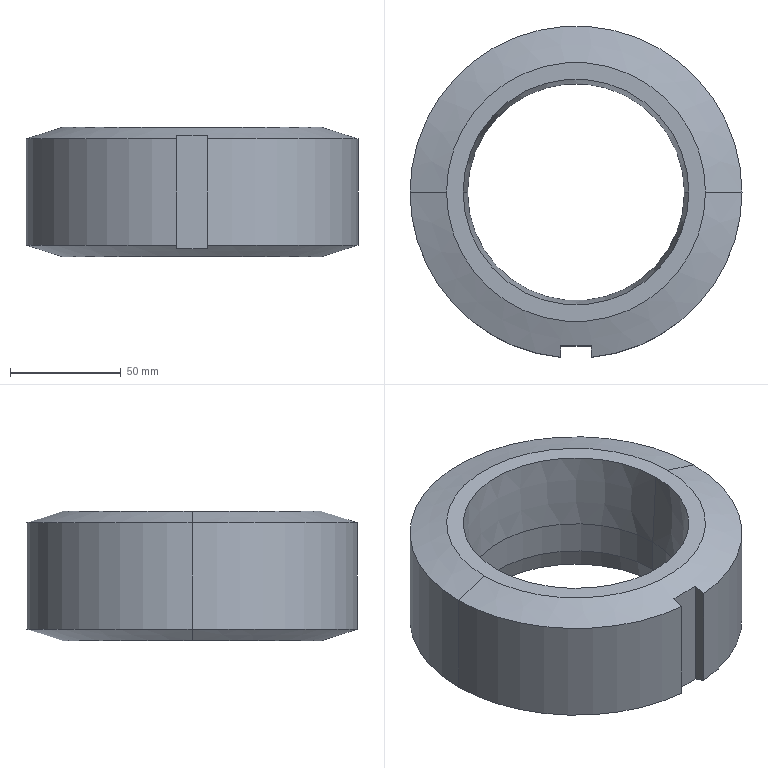Part | SolidWorks | features BaseBody 1, ICE 1 | 1 solid | 18 faces | box 150 x 149.673 x 58.5 mm | volume 537765 mm3 | cone 8 | cylinder 5 | plane 5 | commonest cylinder face diameters 150 x3 98 x2
STEP:
#1=CARTESIAN_POINT('',(570.231,234.744,-789.693));
#2=VERTEX_POINT('',#1);
#3=CARTESIAN_POINT('',(472.231,234.744,-789.693));
#4=VERTEX_POINT('',#3);
#5=CARTESIAN_POINT('',(521.231,234.744,-789.693));
#6=DIRECTION('',(0.,0.,-1.));
#7=DIRECTION('',(-1.,0.,0.));
#8=AXIS2_PLACEMENT_3D('',#5,#6,#7);
#9=CIRCLE('',#8,49.);
#10=EDGE_CURVE('',#2,#4,#9,.T.);
#11=ORIENTED_EDGE('',*,*,#10,.T.);
#12=CARTESIAN_POINT('',(470.231,234.744,-754.693));
#13=VERTEX_POINT('',#12);
#14=CARTESIAN_POINT('',(470.231,234.744,-754.693));
#15=DIRECTION('',(-0.05705,0.,0.9984));
#16=VECTOR('',#15,1000.);
#17=LINE('',#14,#16);
#18=EDGE_CURVE('',#4,#13,#17,.T.);
#19=ORIENTED_EDGE('',*,*,#18,.T.);
#20=CARTESIAN_POINT('',(572.231,234.744,-754.693));
#21=VERTEX_POINT('',#20);
#22=CARTESIAN_POINT('',(521.231,234.744,-754.693));
#23=DIRECTION('',(0.,0.,-1.));
#24=DIRECTION('',(-1.,0.,0.));
#25=AXIS2_PLACEMENT_3D('',#22,#23,#24);
#26=CIRCLE('',#25,51.);
#27=EDGE_CURVE('',#21,#13,#26,.T.);
#28=ORIENTED_EDGE('',*,*,#27,.F.);
#29=CARTESIAN_POINT('',(572.231,234.744,-754.693));
#30=DIRECTION('',(0.05705,0.,0.9984));
#31=VECTOR('',#30,1000.);
#32=LINE('',#29,#31);
#33=EDGE_CURVE('',#2,#21,#32,.T.);
#34=ORIENTED_EDGE('',*,*,#33,.F.);
#35=EDGE_LOOP('',(#11,#19,#28,#34));
#36=FACE_OUTER_BOUND('',#35,.T.);
#37=CARTESIAN_POINT('',(521.231,234.744,-754.693));
#38=DIRECTION('',(0.,0.,1.));
#39=DIRECTION('',(1.,0.,0.));
#40=AXIS2_PLACEMENT_3D('',#37,#38,#39);
#41=CONICAL_SURFACE('',#40,51.,0.05708);
#42=ADVANCED_FACE('',(#36),#41,.F.);
#43=CARTESIAN_POINT('',(462.731,234.744,-754.693));
#44=VERTEX_POINT('',#43);
#45=CARTESIAN_POINT('',(579.731,234.744,-754.693));
#46=VERTEX_POINT('',#45);
#47=CARTESIAN_POINT('',(521.231,234.744,-754.693));
#48=DIRECTION('',(0.,0.,-1.));
#49=DIRECTION('',(-1.,0.,0.));
#50=AXIS2_PLACEMENT_3D('',#47,#48,#49);
#51=CIRCLE('',#50,58.5);
#52=EDGE_CURVE('',#44,#46,#51,.T.);
#53=ORIENTED_EDGE('',*,*,#52,.T.);
#54=CARTESIAN_POINT('',(596.231,234.744,-759.943));
#55=VERTEX_POINT('',#54);
#56=CARTESIAN_POINT('',(579.731,234.744,-754.693));
#57=DIRECTION('',(0.9529,0.,-0.3032));
#58=VECTOR('',#57,1000.);
#59=LINE('',#56,#58);
#60=EDGE_CURVE('',#46,#55,#59,.T.);
#61=ORIENTED_EDGE('',*,*,#60,.T.);
#62=CARTESIAN_POINT('',(446.231,234.744,-759.943));
#63=VERTEX_POINT('',#62);
#64=CARTESIAN_POINT('',(521.231,234.744,-759.943));
#65=DIRECTION('',(0.,0.,-1.));
#66=DIRECTION('',(-1.,0.,0.));
#67=AXIS2_PLACEMENT_3D('',#64,#65,#66);
#68=CIRCLE('',#67,75.);
#69=EDGE_CURVE('',#63,#55,#68,.T.);
#70=ORIENTED_EDGE('',*,*,#69,.F.);
#71=CARTESIAN_POINT('',(462.731,234.744,-754.693));
#72=DIRECTION('',(-0.9529,0.,-0.3032));
#73=VECTOR('',#72,1000.);
#74=LINE('',#71,#73);
#75=EDGE_CURVE('',#44,#63,#74,.T.);
#76=ORIENTED_EDGE('',*,*,#75,.F.);
#77=EDGE_LOOP('',(#53,#61,#70,#76));
#78=FACE_OUTER_BOUND('',#77,.T.);
#79=CARTESIAN_POINT('',(521.231,234.744,-754.693));
#80=DIRECTION('',(0.,0.,-1.));
#81=DIRECTION('',(-1.,0.,0.));
#82=AXIS2_PLACEMENT_3D('',#79,#80,#81);
#83=CONICAL_SURFACE('',#82,58.5,1.263);
#84=ADVANCED_FACE('',(#78),#83,.T.);
#85=CARTESIAN_POINT('',(462.731,234.744,-813.193));
#86=VERTEX_POINT('',#85);
#87=CARTESIAN_POINT('',(579.731,234.744,-813.193));
#88=VERTEX_POINT('',#87);
#89=CARTESIAN_POINT('',(521.231,234.744,-813.193));
#90=DIRECTION('',(0.,0.,-1.));
#91=DIRECTION('',(-1.,0.,0.));
#92=AXIS2_PLACEMENT_3D('',#89,#90,#91);
#93=CIRCLE('',#92,58.5);
#94=EDGE_CURVE('',#86,#88,#93,.T.);
#95=ORIENTED_EDGE('',*,*,#94,.F.);
#96=CARTESIAN_POINT('',(446.231,234.744,-807.943));
#97=VERTEX_POINT('',#96);
#98=CARTESIAN_POINT('',(462.731,234.744,-813.193));
#99=DIRECTION('',(-0.9529,0.,0.3032));
#100=VECTOR('',#99,1000.);
#101=LINE('',#98,#100);
#102=EDGE_CURVE('',#86,#97,#101,.T.);
#103=ORIENTED_EDGE('',*,*,#102,.T.);
#104=CARTESIAN_POINT('',(596.231,234.744,-807.943));
#105=VERTEX_POINT('',#104);
#106=CARTESIAN_POINT('',(521.231,234.744,-807.943));
#107=DIRECTION('',(0.,0.,-1.));
#108=DIRECTION('',(-1.,0.,0.));
#109=AXIS2_PLACEMENT_3D('',#106,#107,#108);
#110=CIRCLE('',#109,75.);
#111=EDGE_CURVE('',#97,#105,#110,.T.);
#112=ORIENTED_EDGE('',*,*,#111,.T.);
#113=CARTESIAN_POINT('',(579.731,234.744,-813.193));
#114=DIRECTION('',(0.9529,0.,0.3032));
#115=VECTOR('',#114,1000.);
#116=LINE('',#113,#115);
#117=EDGE_CURVE('',#88,#105,#116,.T.);
#118=ORIENTED_EDGE('',*,*,#117,.F.);
#119=EDGE_LOOP('',(#95,#103,#112,#118));
#120=FACE_OUTER_BOUND('',#119,.T.);
#121=CARTESIAN_POINT('',(521.231,234.744,-813.193));
#122=DIRECTION('',(0.,0.,1.));
#123=DIRECTION('',(1.,0.,0.));
#124=AXIS2_PLACEMENT_3D('',#121,#122,#123);
#125=CONICAL_SURFACE('',#124,58.5,1.263);
#126=ADVANCED_FACE('',(#120),#125,.T.);
#127=ORIENTED_EDGE('',*,*,#111,.F.);
#128=CARTESIAN_POINT('',(446.231,234.744,-814.693));
#129=DIRECTION('',(0.,0.,1.));
#130=VECTOR('',#129,1000.);
#131=LINE('',#128,#130);
#132=EDGE_CURVE('',#97,#63,#131,.T.);
#133=ORIENTED_EDGE('',*,*,#132,.T.);
#134=ORIENTED_EDGE('',*,*,#69,.T.);
#135=CARTESIAN_POINT('',(596.231,234.744,-814.693));
#136=DIRECTION('',(0.,0.,1.));
#137=VECTOR('',#136,1000.);
#138=LINE('',#135,#137);
#139=EDGE_CURVE('',#105,#55,#138,.T.);
#140=ORIENTED_EDGE('',*,*,#139,.F.);
#141=EDGE_LOOP('',(#127,#133,#134,#140));
#142=FACE_OUTER_BOUND('',#141,.T.);
#143=CARTESIAN_POINT('',(521.231,234.744,-814.693));
#144=DIRECTION('',(0.,0.,1.));
#145=DIRECTION('',(1.,0.,0.));
#146=AXIS2_PLACEMENT_3D('',#143,#144,#145);
#147=CYLINDRICAL_SURFACE('',#146,75.);
#148=ADVANCED_FACE('',(#142),#147,.T.);
#149=CARTESIAN_POINT('',(528.231,160.071,-807.943));
#150=VERTEX_POINT('',#149);
#151=CARTESIAN_POINT('',(521.231,234.744,-807.943));
#152=DIRECTION('',(0.,0.,-1.));
#153=DIRECTION('',(-1.,0.,0.));
#154=AXIS2_PLACEMENT_3D('',#151,#152,#153);
#155=CIRCLE('',#154,75.);
#156=EDGE_CURVE('',#105,#150,#155,.T.);
#157=ORIENTED_EDGE('',*,*,#156,.F.);
#158=ORIENTED_EDGE('',*,*,#139,.T.);
#159=CARTESIAN_POINT('',(528.231,160.071,-759.943));
#160=VERTEX_POINT('',#159);
#161=CARTESIAN_POINT('',(521.231,234.744,-759.943));
#162=DIRECTION('',(0.,0.,-1.));
#163=DIRECTION('',(-1.,0.,0.));
#164=AXIS2_PLACEMENT_3D('',#161,#162,#163);
#165=CIRCLE('',#164,75.);
#166=EDGE_CURVE('',#55,#160,#165,.T.);
#167=ORIENTED_EDGE('',*,*,#166,.T.);
#168=CARTESIAN_POINT('',(528.231,160.071,-814.693));
#169=DIRECTION('',(0.,0.,-1.));
#170=VECTOR('',#169,1000.);
#171=LINE('',#168,#170);
#172=EDGE_CURVE('',#160,#150,#171,.T.);
#173=ORIENTED_EDGE('',*,*,#172,.T.);
#174=EDGE_LOOP('',(#157,#158,#167,#173));
#175=FACE_OUTER_BOUND('',#174,.T.);
#176=CARTESIAN_POINT('',(521.231,234.744,-814.693));
#177=DIRECTION('',(0.,0.,1.));
#178=DIRECTION('',(1.,0.,0.));
#179=AXIS2_PLACEMENT_3D('',#176,#177,#178);
#180=CYLINDRICAL_SURFACE('',#179,75.);
#181=ADVANCED_FACE('',(#175),#180,.T.);
#182=ORIENTED_EDGE('',*,*,#10,.F.);
#183=CARTESIAN_POINT('',(570.231,234.744,-804.693));
#184=VERTEX_POINT('',#183);
#185=CARTESIAN_POINT('',(570.231,234.744,-754.693));
#186=DIRECTION('',(0.,0.,-1.));
#187=VECTOR('',#186,1000.);
#188=LINE('',#185,#187);
#189=EDGE_CURVE('',#2,#184,#188,.T.);
#190=ORIENTED_EDGE('',*,*,#189,.T.);
#191=CARTESIAN_POINT('',(472.231,234.744,-804.693));
#192=VERTEX_POINT('',#191);
#193=CARTESIAN_POINT('',(521.231,234.744,-804.693));
#194=DIRECTION('',(0.,0.,-1.));
#195=DIRECTION('',(-1.,0.,0.));
#196=AXIS2_PLACEMENT_3D('',#193,#194,#195);
#197=CIRCLE('',#196,49.);
#198=EDGE_CURVE('',#184,#192,#197,.T.);
#199=ORIENTED_EDGE('',*,*,#198,.T.);
#200=CARTESIAN_POINT('',(472.231,234.744,-754.693));
#201=DIRECTION('',(0.,0.,-1.));
#202=VECTOR('',#201,1000.);
#203=LINE('',#200,#202);
#204=EDGE_CURVE('',#4,#192,#203,.T.);
#205=ORIENTED_EDGE('',*,*,#204,.F.);
#206=EDGE_LOOP('',(#182,#190,#199,#205));
#207=FACE_OUTER_BOUND('',#206,.T.);
#208=CARTESIAN_POINT('',(521.231,234.744,-754.693));
#209=DIRECTION('',(0.,0.,-1.));
#210=DIRECTION('',(-1.,0.,0.));
#211=AXIS2_PLACEMENT_3D('',#208,#209,#210);
#212=CYLINDRICAL_SURFACE('',#211,49.);
#213=ADVANCED_FACE('',(#207),#212,.F.);
#214=ORIENTED_EDGE('',*,*,#198,.F.);
#215=CARTESIAN_POINT('',(571.931,234.744,-813.193));
#216=VERTEX_POINT('',#215);
#217=CARTESIAN_POINT('',(570.231,234.744,-804.693));
#218=DIRECTION('',(0.1961,0.,-0.9806));
#219=VECTOR('',#218,1000.);
#220=LINE('',#217,#219);
#221=EDGE_CURVE('',#184,#216,#220,.T.);
#222=ORIENTED_EDGE('',*,*,#221,.T.);
#223=CARTESIAN_POINT('',(470.531,234.744,-813.193));
#224=VERTEX_POINT('',#223);
#225=CARTESIAN_POINT('',(521.231,234.744,-813.193));
#226=DIRECTION('',(0.,0.,-1.));
#227=DIRECTION('',(-1.,0.,0.));
#228=AXIS2_PLACEMENT_3D('',#225,#226,#227);
#229=CIRCLE('',#228,50.7);
#230=EDGE_CURVE('',#216,#224,#229,.T.);
#231=ORIENTED_EDGE('',*,*,#230,.T.);
#232=CARTESIAN_POINT('',(472.231,234.744,-804.693));
#233=DIRECTION('',(-0.1961,0.,-0.9806));
#234=VECTOR('',#233,1000.);
#235=LINE('',#232,#234);
#236=EDGE_CURVE('',#192,#224,#235,.T.);
#237=ORIENTED_EDGE('',*,*,#236,.F.);
#238=EDGE_LOOP('',(#214,#222,#231,#237));
#239=FACE_OUTER_BOUND('',#238,.T.);
#240=CARTESIAN_POINT('',(521.231,234.744,-804.693));
#241=DIRECTION('',(0.,0.,-1.));
#242=DIRECTION('',(-1.,0.,0.));
#243=AXIS2_PLACEMENT_3D('',#240,#241,#242);
#244=CONICAL_SURFACE('',#243,49.,0.1974);
#245=ADVANCED_FACE('',(#239),#244,.F.);
#246=ORIENTED_EDGE('',*,*,#221,.F.);
#247=CARTESIAN_POINT('',(521.231,234.744,-804.693));
#248=DIRECTION('',(0.,0.,-1.));
#249=DIRECTION('',(-1.,0.,0.));
#250=AXIS2_PLACEMENT_3D('',#247,#248,#249);
#251=CIRCLE('',#250,49.);
#252=EDGE_CURVE('',#192,#184,#251,.T.);
#253=ORIENTED_EDGE('',*,*,#252,.F.);
#254=ORIENTED_EDGE('',*,*,#236,.T.);
#255=CARTESIAN_POINT('',(521.231,234.744,-813.193));
#256=DIRECTION('',(0.,0.,-1.));
#257=DIRECTION('',(-1.,0.,0.));
#258=AXIS2_PLACEMENT_3D('',#255,#256,#257);
#259=CIRCLE('',#258,50.7);
#260=EDGE_CURVE('',#224,#216,#259,.T.);
#261=ORIENTED_EDGE('',*,*,#260,.T.);
#262=EDGE_LOOP('',(#246,#253,#254,#261));
#263=FACE_OUTER_BOUND('',#262,.T.);
#264=CARTESIAN_POINT('',(521.231,234.744,-804.693));
#265=DIRECTION('',(0.,0.,-1.));
#266=DIRECTION('',(-1.,0.,0.));
#267=AXIS2_PLACEMENT_3D('',#264,#265,#266);
#268=CONICAL_SURFACE('',#267,49.,0.1974);
#269=ADVANCED_FACE('',(#263),#268,.F.);
#270=ORIENTED_EDGE('',*,*,#189,.F.);
#271=CARTESIAN_POINT('',(521.231,234.744,-789.693));
#272=DIRECTION('',(0.,0.,-1.));
#273=DIRECTION('',(-1.,0.,0.));
#274=AXIS2_PLACEMENT_3D('',#271,#272,#273);
#275=CIRCLE('',#274,49.);
#276=EDGE_CURVE('',#4,#2,#275,.T.);
#277=ORIENTED_EDGE('',*,*,#276,.F.);
#278=ORIENTED_EDGE('',*,*,#204,.T.);
#279=ORIENTED_EDGE('',*,*,#252,.T.);
#280=EDGE_LOOP('',(#270,#277,#278,#279));
#281=FACE_OUTER_BOUND('',#280,.T.);
#282=CARTESIAN_POINT('',(521.231,234.744,-754.693));
#283=DIRECTION('',(0.,0.,-1.));
#284=DIRECTION('',(-1.,0.,0.));
#285=AXIS2_PLACEMENT_3D('',#282,#283,#284);
#286=CYLINDRICAL_SURFACE('',#285,49.);
#287=ADVANCED_FACE('',(#281),#286,.F.);
#288=ORIENTED_EDGE('',*,*,#27,.T.);
#289=CARTESIAN_POINT('',(521.231,234.744,-754.693));
#290=DIRECTION('',(0.,0.,-1.));
#291=DIRECTION('',(-1.,0.,0.));
#292=AXIS2_PLACEMENT_3D('',#289,#290,#291);
#293=CIRCLE('',#292,51.);
#294=EDGE_CURVE('',#13,#21,#293,.T.);
#295=ORIENTED_EDGE('',*,*,#294,.T.);
#296=EDGE_LOOP('',(#288,#295));
#297=FACE_BOUND('',#296,.T.);
#298=ORIENTED_EDGE('',*,*,#52,.F.);
#299=CARTESIAN_POINT('',(521.231,234.744,-754.693));
#300=DIRECTION('',(0.,0.,-1.));
#301=DIRECTION('',(-1.,0.,0.));
#302=AXIS2_PLACEMENT_3D('',#299,#300,#301);
#303=CIRCLE('',#302,58.5);
#304=EDGE_CURVE('',#46,#44,#303,.T.);
#305=ORIENTED_EDGE('',*,*,#304,.F.);
#306=EDGE_LOOP('',(#298,#305));
#307=FACE_OUTER_BOUND('',#306,.T.);
#308=CARTESIAN_POINT('',(521.231,234.744,-754.693));
#309=DIRECTION('',(0.,0.,-1.));
#310=DIRECTION('',(-1.,0.,0.));
#311=AXIS2_PLACEMENT_3D('',#308,#309,#310);
#312=PLANE('',#311);
#313=ADVANCED_FACE('',(#297,#307),#312,.F.);
#314=ORIENTED_EDGE('',*,*,#132,.F.);
#315=CARTESIAN_POINT('',(514.231,160.071,-807.943));
#316=VERTEX_POINT('',#315);
#317=CARTESIAN_POINT('',(521.231,234.744,-807.943));
#318=DIRECTION('',(0.,0.,-1.));
#319=DIRECTION('',(-1.,0.,0.));
#320=AXIS2_PLACEMENT_3D('',#317,#318,#319);
#321=CIRCLE('',#320,75.);
#322=EDGE_CURVE('',#316,#97,#321,.T.);
#323=ORIENTED_EDGE('',*,*,#322,.F.);
#324=CARTESIAN_POINT('',(514.231,160.071,-759.943));
#325=VERTEX_POINT('',#324);
#326=CARTESIAN_POINT('',(514.231,160.071,-814.693));
#327=DIRECTION('',(0.,0.,1.));
#328=VECTOR('',#327,1000.);
#329=LINE('',#326,#328);
#330=EDGE_CURVE('',#316,#325,#329,.T.);
#331=ORIENTED_EDGE('',*,*,#330,.T.);
#332=CARTESIAN_POINT('',(521.231,234.744,-759.943));
#333=DIRECTION('',(0.,0.,-1.));
#334=DIRECTION('',(-1.,0.,0.));
#335=AXIS2_PLACEMENT_3D('',#332,#333,#334);
#336=CIRCLE('',#335,75.);
#337=EDGE_CURVE('',#325,#63,#336,.T.);
#338=ORIENTED_EDGE('',*,*,#337,.T.);
#339=EDGE_LOOP('',(#314,#323,#331,#338));
#340=FACE_OUTER_BOUND('',#339,.T.);
#341=CARTESIAN_POINT('',(521.231,234.744,-814.693));
#342=DIRECTION('',(0.,0.,1.));
#343=DIRECTION('',(1.,0.,0.));
#344=AXIS2_PLACEMENT_3D('',#341,#342,#343);
#345=CYLINDRICAL_SURFACE('',#344,75.);
#346=ADVANCED_FACE('',(#340),#345,.T.);
#347=ORIENTED_EDGE('',*,*,#102,.F.);
#348=CARTESIAN_POINT('',(521.231,234.744,-813.193));
#349=DIRECTION('',(0.,0.,-1.));
#350=DIRECTION('',(-1.,0.,0.));
#351=AXIS2_PLACEMENT_3D('',#348,#349,#350);
#352=CIRCLE('',#351,58.5);
#353=EDGE_CURVE('',#88,#86,#352,.T.);
#354=ORIENTED_EDGE('',*,*,#353,.F.);
#355=ORIENTED_EDGE('',*,*,#117,.T.);
#356=ORIENTED_EDGE('',*,*,#156,.T.);
#357=CARTESIAN_POINT('',(528.231,165.244,-809.581));
#358=VERTEX_POINT('',#357);
#359=CARTESIAN_POINT('',(528.231,165.244,-809.581));
#360=CARTESIAN_POINT('',(528.231,163.692,-809.09));
#361=CARTESIAN_POINT('',(528.231,162.14,-808.598));
#362=CARTESIAN_POINT('',(528.231,160.588,-808.107));
#363=CARTESIAN_POINT('',(528.231,160.415,-808.052));
#364=CARTESIAN_POINT('',(528.231,160.243,-807.997));
#365=CARTESIAN_POINT('',(528.231,160.071,-807.943));
#366=B_SPLINE_CURVE_WITH_KNOTS('',3,(#359,#360,#361,#362,#363,#364,#365),.UNSPECIFIED.,.F.,.F.,(4,3,4),(0.008941,0.01383,0.01437),.UNSPECIFIED.);
#367=EDGE_CURVE('',#358,#150,#366,.T.);
#368=ORIENTED_EDGE('',*,*,#367,.F.);
#369=CARTESIAN_POINT('',(514.231,165.244,-809.581));
#370=VERTEX_POINT('',#369);
#371=CARTESIAN_POINT('',(514.231,165.244,-809.581));
#372=CARTESIAN_POINT('',(516.561,165.244,-809.655));
#373=CARTESIAN_POINT('',(518.893,165.244,-809.693));
#374=CARTESIAN_POINT('',(523.56,165.244,-809.693));
#375=CARTESIAN_POINT('',(525.896,165.244,-809.656));
#376=CARTESIAN_POINT('',(528.231,165.244,-809.581));
#377=B_SPLINE_CURVE_WITH_KNOTS('',3,(#371,#372,#373,#374,#375,#376),.UNSPECIFIED.,.F.,.F.,(4,2,4),(0.01756,0.02456,0.03155),.UNSPECIFIED.);
#378=EDGE_CURVE('',#370,#358,#377,.T.);
#379=ORIENTED_EDGE('',*,*,#378,.F.);
#380=CARTESIAN_POINT('',(514.231,160.071,-807.943));
#381=CARTESIAN_POINT('',(514.231,160.243,-807.997));
#382=CARTESIAN_POINT('',(514.231,160.415,-808.052));
#383=CARTESIAN_POINT('',(514.231,160.588,-808.107));
#384=CARTESIAN_POINT('',(514.231,162.14,-808.598));
#385=CARTESIAN_POINT('',(514.231,163.692,-809.09));
#386=CARTESIAN_POINT('',(514.231,165.244,-809.581));
#387=B_SPLINE_CURVE_WITH_KNOTS('',3,(#380,#381,#382,#383,#384,#385,#386),.UNSPECIFIED.,.F.,.F.,(4,3,4),(0.01328,0.01383,0.01871),.UNSPECIFIED.);
#388=EDGE_CURVE('',#316,#370,#387,.T.);
#389=ORIENTED_EDGE('',*,*,#388,.F.);
#390=ORIENTED_EDGE('',*,*,#322,.T.);
#391=EDGE_LOOP('',(#347,#354,#355,#356,#368,#379,#389,#390));
#392=FACE_OUTER_BOUND('',#391,.T.);
#393=CARTESIAN_POINT('',(521.231,234.744,-813.193));
#394=DIRECTION('',(0.,0.,1.));
#395=DIRECTION('',(1.,0.,0.));
#396=AXIS2_PLACEMENT_3D('',#393,#394,#395);
#397=CONICAL_SURFACE('',#396,58.5,1.263);
#398=ADVANCED_FACE('',(#392),#397,.T.);
#399=ORIENTED_EDGE('',*,*,#60,.F.);
#400=ORIENTED_EDGE('',*,*,#304,.T.);
#401=ORIENTED_EDGE('',*,*,#75,.T.);
#402=ORIENTED_EDGE('',*,*,#337,.F.);
#403=CARTESIAN_POINT('',(514.231,165.244,-758.305));
#404=VERTEX_POINT('',#403);
#405=CARTESIAN_POINT('',(514.231,160.071,-759.943));
#406=CARTESIAN_POINT('',(514.231,160.243,-759.888));
#407=CARTESIAN_POINT('',(514.231,160.415,-759.834));
#408=CARTESIAN_POINT('',(514.231,160.588,-759.779));
#409=CARTESIAN_POINT('',(514.231,162.14,-759.288));
#410=CARTESIAN_POINT('',(514.231,163.692,-758.796));
#411=CARTESIAN_POINT('',(514.231,165.244,-758.305));
#412=B_SPLINE_CURVE_WITH_KNOTS('',3,(#405,#406,#407,#408,#409,#410,#411),.UNSPECIFIED.,.F.,.F.,(4,3,4),(0.01328,0.01383,0.01871),.UNSPECIFIED.);
#413=EDGE_CURVE('',#325,#404,#412,.T.);
#414=ORIENTED_EDGE('',*,*,#413,.T.);
#415=CARTESIAN_POINT('',(528.231,165.244,-758.305));
#416=VERTEX_POINT('',#415);
#417=CARTESIAN_POINT('',(514.231,165.244,-758.305));
#418=CARTESIAN_POINT('',(516.561,165.244,-758.231));
#419=CARTESIAN_POINT('',(518.893,165.244,-758.193));
#420=CARTESIAN_POINT('',(523.56,165.244,-758.193));
#421=CARTESIAN_POINT('',(525.896,165.244,-758.23));
#422=CARTESIAN_POINT('',(528.231,165.244,-758.305));
#423=B_SPLINE_CURVE_WITH_KNOTS('',3,(#417,#418,#419,#420,#421,#422),.UNSPECIFIED.,.F.,.F.,(4,2,4),(0.01756,0.02456,0.03155),.UNSPECIFIED.);
#424=EDGE_CURVE('',#404,#416,#423,.T.);
#425=ORIENTED_EDGE('',*,*,#424,.T.);
#426=CARTESIAN_POINT('',(528.231,165.244,-758.305));
#427=CARTESIAN_POINT('',(528.231,163.692,-758.796));
#428=CARTESIAN_POINT('',(528.231,162.14,-759.288));
#429=CARTESIAN_POINT('',(528.231,160.588,-759.779));
#430=CARTESIAN_POINT('',(528.231,160.415,-759.834));
#431=CARTESIAN_POINT('',(528.231,160.243,-759.888));
#432=CARTESIAN_POINT('',(528.231,160.071,-759.943));
#433=B_SPLINE_CURVE_WITH_KNOTS('',3,(#426,#427,#428,#429,#430,#431,#432),.UNSPECIFIED.,.F.,.F.,(4,3,4),(0.008941,0.01383,0.01437),.UNSPECIFIED.);
#434=EDGE_CURVE('',#416,#160,#433,.T.);
#435=ORIENTED_EDGE('',*,*,#434,.T.);
#436=ORIENTED_EDGE('',*,*,#166,.F.);
#437=EDGE_LOOP('',(#399,#400,#401,#402,#414,#425,#435,#436));
#438=FACE_OUTER_BOUND('',#437,.T.);
#439=CARTESIAN_POINT('',(521.231,234.744,-754.693));
#440=DIRECTION('',(0.,0.,-1.));
#441=DIRECTION('',(-1.,0.,0.));
#442=AXIS2_PLACEMENT_3D('',#439,#440,#441);
#443=CONICAL_SURFACE('',#442,58.5,1.263);
#444=ADVANCED_FACE('',(#438),#443,.T.);
#445=ORIENTED_EDGE('',*,*,#18,.F.);
#446=ORIENTED_EDGE('',*,*,#276,.T.);
#447=ORIENTED_EDGE('',*,*,#33,.T.);
#448=ORIENTED_EDGE('',*,*,#294,.F.);
#449=EDGE_LOOP('',(#445,#446,#447,#448));
#450=FACE_OUTER_BOUND('',#449,.T.);
#451=CARTESIAN_POINT('',(521.231,234.744,-754.693));
#452=DIRECTION('',(0.,0.,1.));
#453=DIRECTION('',(1.,0.,0.));
#454=AXIS2_PLACEMENT_3D('',#451,#452,#453);
#455=CONICAL_SURFACE('',#454,51.,0.05708);
#456=ADVANCED_FACE('',(#450),#455,.F.);
#457=ORIENTED_EDGE('',*,*,#378,.T.);
#458=CARTESIAN_POINT('',(528.231,165.244,-1254.693));
#459=DIRECTION('',(0.,0.,1.));
#460=VECTOR('',#459,1000.);
#461=LINE('',#458,#460);
#462=EDGE_CURVE('',#358,#416,#461,.T.);
#463=ORIENTED_EDGE('',*,*,#462,.T.);
#464=ORIENTED_EDGE('',*,*,#424,.F.);
#465=CARTESIAN_POINT('',(514.231,165.244,-1254.693));
#466=DIRECTION('',(0.,0.,1.));
#467=VECTOR('',#466,1000.);
#468=LINE('',#465,#467);
#469=EDGE_CURVE('',#370,#404,#468,.T.);
#470=ORIENTED_EDGE('',*,*,#469,.F.);
#471=EDGE_LOOP('',(#457,#463,#464,#470));
#472=FACE_OUTER_BOUND('',#471,.T.);
#473=CARTESIAN_POINT('',(528.231,165.244,-1254.693));
#474=DIRECTION('',(0.,1.,0.));
#475=DIRECTION('',(0.,0.,-1.));
#476=AXIS2_PLACEMENT_3D('',#473,#474,#475);
#477=PLANE('',#476);
#478=ADVANCED_FACE('',(#472),#477,.F.);
#479=ORIENTED_EDGE('',*,*,#367,.T.);
#480=ORIENTED_EDGE('',*,*,#172,.F.);
#481=ORIENTED_EDGE('',*,*,#434,.F.);
#482=ORIENTED_EDGE('',*,*,#462,.F.);
#483=EDGE_LOOP('',(#479,#480,#481,#482));
#484=FACE_OUTER_BOUND('',#483,.T.);
#485=CARTESIAN_POINT('',(528.231,153.998,-1254.693));
#486=DIRECTION('',(1.,0.,0.));
#487=DIRECTION('',(0.,0.,-1.));
#488=AXIS2_PLACEMENT_3D('',#485,#486,#487);
#489=PLANE('',#488);
#490=ADVANCED_FACE('',(#484),#489,.F.);
#491=ORIENTED_EDGE('',*,*,#388,.T.);
#492=ORIENTED_EDGE('',*,*,#469,.T.);
#493=ORIENTED_EDGE('',*,*,#413,.F.);
#494=ORIENTED_EDGE('',*,*,#330,.F.);
#495=EDGE_LOOP('',(#491,#492,#493,#494));
#496=FACE_OUTER_BOUND('',#495,.T.);
#497=CARTESIAN_POINT('',(514.231,165.244,-1254.693));
#498=DIRECTION('',(-1.,0.,0.));
#499=DIRECTION('',(0.,0.,1.));
#500=AXIS2_PLACEMENT_3D('',#497,#498,#499);
#501=PLANE('',#500);
#502=ADVANCED_FACE('',(#496),#501,.F.);
#503=ORIENTED_EDGE('',*,*,#260,.F.);
#504=ORIENTED_EDGE('',*,*,#230,.F.);
#505=EDGE_LOOP('',(#503,#504));
#506=FACE_BOUND('',#505,.T.);
#507=ORIENTED_EDGE('',*,*,#353,.T.);
#508=ORIENTED_EDGE('',*,*,#94,.T.);
#509=EDGE_LOOP('',(#507,#508));
#510=FACE_OUTER_BOUND('',#509,.T.);
#511=CARTESIAN_POINT('',(521.231,234.744,-813.193));
#512=DIRECTION('',(0.,0.,-1.));
#513=DIRECTION('',(-1.,0.,0.));
#514=AXIS2_PLACEMENT_3D('',#511,#512,#513);
#515=PLANE('',#514);
#516=ADVANCED_FACE('',(#506,#510),#515,.T.);
#517=CLOSED_SHELL('',(#42,#84,#126,#148,#181,#213,#245,#269,#287,#313,#346,#398,#444,#456,#478,#490,#502,#516));
#518=MANIFOLD_SOLID_BREP('',#517);
#519=CARTESIAN_POINT('',(0.,0.,0.));
#520=DIRECTION('',(0.,0.,1.));
#521=DIRECTION('',(1.,0.,0.));
#522=AXIS2_PLACEMENT_3D('',#519,#520,#521);
#523=(LENGTH_UNIT()NAMED_UNIT(*)SI_UNIT(.MILLI.,.METRE.));
#524=UNCERTAINTY_MEASURE_WITH_UNIT(LENGTH_MEASURE(0.00001),#523,'','');
#525=(NAMED_UNIT(*)PLANE_ANGLE_UNIT()SI_UNIT($,.RADIAN.));
#526=(NAMED_UNIT(*)SI_UNIT($,.STERADIAN.)SOLID_ANGLE_UNIT());
#527=(GEOMETRIC_REPRESENTATION_CONTEXT(3)GLOBAL_UNCERTAINTY_ASSIGNED_CONTEXT((#524))GLOBAL_UNIT_ASSIGNED_CONTEXT((#523,#525,#526))REPRESENTATION_CONTEXT('',''));
#528=ADVANCED_BREP_SHAPE_REPRESENTATION('',(#518,#522),#527);